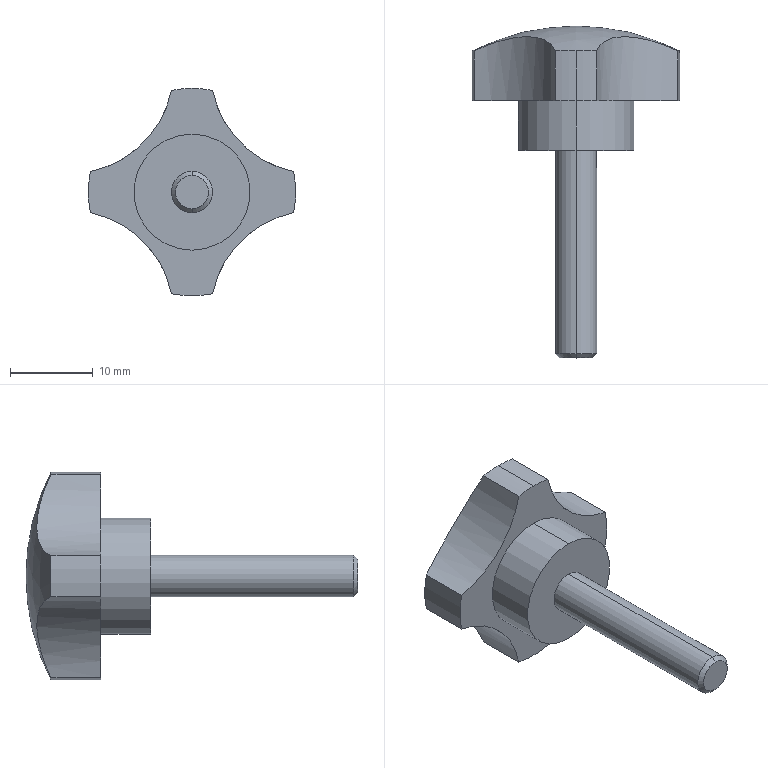Part | NX | features BREP 1 | 1 solid | 19 faces | box 25 x 40 x 25 mm | volume 4055 mm3 | cylinder 13 | plane 3 | cone 2 | sphere 1 | commonest cylinder face diameters 25 x9 5 x2 14 x2
STEP:
#1=CARTESIAN_POINT('',(12.252,12.,-2.48));
#2=VERTEX_POINT('',#1);
#3=CARTESIAN_POINT('',(12.252,12.,2.48));
#4=VERTEX_POINT('',#3);
#5=CARTESIAN_POINT('',(0.,12.,0.));
#6=DIRECTION('',(0.,-1.,0.));
#7=DIRECTION('',(0.,0.,1.));
#8=AXIS2_PLACEMENT_3D('',#5,#6,#7);
#9=CIRCLE('',#8,12.5);
#10=EDGE_CURVE('',#2,#4,#9,.T.);
#11=ORIENTED_EDGE('',*,*,#10,.F.);
#12=CARTESIAN_POINT('',(2.48,12.,-12.252));
#13=VERTEX_POINT('',#12);
#14=CARTESIAN_POINT('',(2.48,12.,-12.252));
#15=CARTESIAN_POINT('',(2.715,12.557,-11.089));
#16=CARTESIAN_POINT('',(3.495,13.393,-8.858));
#17=CARTESIAN_POINT('',(5.756,13.868,-5.744));
#18=CARTESIAN_POINT('',(8.866,13.39,-3.492));
#19=CARTESIAN_POINT('',(11.091,12.555,-2.715));
#20=CARTESIAN_POINT('',(12.252,12.,-2.48));
#21=B_SPLINE_CURVE_WITH_KNOTS('',3,(#14,#15,#16,#17,#18,#19,#20),.UNSPECIFIED.,.F.,.F.,(4,1,1,1,4),(0.,0.25,0.5,0.75,1.),.UNSPECIFIED.);
#22=EDGE_CURVE('',#2,#13,#21,.F.);
#23=ORIENTED_EDGE('',*,*,#22,.T.);
#24=CARTESIAN_POINT('',(-2.48,12.,-12.252));
#25=VERTEX_POINT('',#24);
#26=CARTESIAN_POINT('',(0.,12.,0.));
#27=DIRECTION('',(0.,-1.,0.));
#28=DIRECTION('',(0.,0.,1.));
#29=AXIS2_PLACEMENT_3D('',#26,#27,#28);
#30=CIRCLE('',#29,12.5);
#31=EDGE_CURVE('',#25,#13,#30,.T.);
#32=ORIENTED_EDGE('',*,*,#31,.F.);
#33=CARTESIAN_POINT('',(-12.252,12.,-2.48));
#34=VERTEX_POINT('',#33);
#35=CARTESIAN_POINT('',(-12.252,12.,-2.48));
#36=CARTESIAN_POINT('',(-11.089,12.557,-2.715));
#37=CARTESIAN_POINT('',(-8.858,13.393,-3.495));
#38=CARTESIAN_POINT('',(-5.744,13.868,-5.756));
#39=CARTESIAN_POINT('',(-3.492,13.39,-8.866));
#40=CARTESIAN_POINT('',(-2.715,12.555,-11.091));
#41=CARTESIAN_POINT('',(-2.48,12.,-12.252));
#42=B_SPLINE_CURVE_WITH_KNOTS('',3,(#35,#36,#37,#38,#39,#40,#41),.UNSPECIFIED.,.F.,.F.,(4,1,1,1,4),(0.,0.25,0.5,0.75,1.),.UNSPECIFIED.);
#43=EDGE_CURVE('',#25,#34,#42,.F.);
#44=ORIENTED_EDGE('',*,*,#43,.T.);
#45=CARTESIAN_POINT('',(-12.252,12.,2.48));
#46=VERTEX_POINT('',#45);
#47=CARTESIAN_POINT('',(0.,12.,0.));
#48=DIRECTION('',(0.,-1.,0.));
#49=DIRECTION('',(0.,0.,1.));
#50=AXIS2_PLACEMENT_3D('',#47,#48,#49);
#51=CIRCLE('',#50,12.5);
#52=EDGE_CURVE('',#46,#34,#51,.T.);
#53=ORIENTED_EDGE('',*,*,#52,.F.);
#54=CARTESIAN_POINT('',(-2.48,12.,12.252));
#55=VERTEX_POINT('',#54);
#56=CARTESIAN_POINT('',(-2.48,12.,12.252));
#57=CARTESIAN_POINT('',(-2.715,12.557,11.089));
#58=CARTESIAN_POINT('',(-3.495,13.393,8.858));
#59=CARTESIAN_POINT('',(-5.756,13.868,5.744));
#60=CARTESIAN_POINT('',(-8.866,13.39,3.492));
#61=CARTESIAN_POINT('',(-11.091,12.555,2.715));
#62=CARTESIAN_POINT('',(-12.252,12.,2.48));
#63=B_SPLINE_CURVE_WITH_KNOTS('',3,(#56,#57,#58,#59,#60,#61,#62),.UNSPECIFIED.,.F.,.F.,(4,1,1,1,4),(0.,0.25,0.5,0.75,1.),.UNSPECIFIED.);
#64=EDGE_CURVE('',#46,#55,#63,.F.);
#65=ORIENTED_EDGE('',*,*,#64,.T.);
#66=CARTESIAN_POINT('',(0.,12.,12.5));
#67=VERTEX_POINT('',#66);
#68=CARTESIAN_POINT('',(0.,12.,0.));
#69=DIRECTION('',(0.,-1.,0.));
#70=DIRECTION('',(0.,0.,1.));
#71=AXIS2_PLACEMENT_3D('',#68,#69,#70);
#72=CIRCLE('',#71,12.5);
#73=EDGE_CURVE('',#67,#55,#72,.T.);
#74=ORIENTED_EDGE('',*,*,#73,.F.);
#75=CARTESIAN_POINT('',(2.48,12.,12.252));
#76=VERTEX_POINT('',#75);
#77=CARTESIAN_POINT('',(0.,12.,0.));
#78=DIRECTION('',(0.,-1.,0.));
#79=DIRECTION('',(0.,0.,1.));
#80=AXIS2_PLACEMENT_3D('',#77,#78,#79);
#81=CIRCLE('',#80,12.5);
#82=EDGE_CURVE('',#76,#67,#81,.T.);
#83=ORIENTED_EDGE('',*,*,#82,.F.);
#84=CARTESIAN_POINT('',(12.252,12.,2.48));
#85=CARTESIAN_POINT('',(11.089,12.557,2.715));
#86=CARTESIAN_POINT('',(8.858,13.393,3.495));
#87=CARTESIAN_POINT('',(5.744,13.868,5.756));
#88=CARTESIAN_POINT('',(3.492,13.39,8.866));
#89=CARTESIAN_POINT('',(2.715,12.555,11.091));
#90=CARTESIAN_POINT('',(2.48,12.,12.252));
#91=B_SPLINE_CURVE_WITH_KNOTS('',3,(#84,#85,#86,#87,#88,#89,#90),.UNSPECIFIED.,.F.,.F.,(4,1,1,1,4),(0.,0.25,0.5,0.75,1.),.UNSPECIFIED.);
#92=EDGE_CURVE('',#76,#4,#91,.F.);
#93=ORIENTED_EDGE('',*,*,#92,.T.);
#94=EDGE_LOOP('',(#11,#23,#32,#44,#53,#65,#74,#83,#93));
#95=FACE_BOUND('',#94,.T.);
#96=CARTESIAN_POINT('',(0.,-12.542,0.));
#97=DIRECTION('',(1.,0.,0.));
#98=DIRECTION('',(0.,0.,-1.));
#99=AXIS2_PLACEMENT_3D('',#96,#97,#98);
#100=SPHERICAL_SURFACE('',#99,27.542);
#101=ADVANCED_FACE('',(#95),#100,.T.);
#102=CARTESIAN_POINT('',(-12.252,6.,2.48));
#103=VERTEX_POINT('',#102);
#104=CARTESIAN_POINT('',(-12.252,25.,2.48));
#105=DIRECTION('',(0.,1.,0.));
#106=VECTOR('',#105,1000.);
#107=LINE('',#104,#106);
#108=EDGE_CURVE('',#103,#46,#107,.T.);
#109=ORIENTED_EDGE('',*,*,#108,.T.);
#110=ORIENTED_EDGE('',*,*,#52,.T.);
#111=CARTESIAN_POINT('',(-12.252,6.,-2.48));
#112=VERTEX_POINT('',#111);
#113=CARTESIAN_POINT('',(-12.252,25.,-2.48));
#114=DIRECTION('',(0.,-1.,0.));
#115=VECTOR('',#114,1000.);
#116=LINE('',#113,#115);
#117=EDGE_CURVE('',#34,#112,#116,.T.);
#118=ORIENTED_EDGE('',*,*,#117,.T.);
#119=CARTESIAN_POINT('',(0.,6.,0.));
#120=DIRECTION('',(0.,1.,0.));
#121=DIRECTION('',(0.,0.,1.));
#122=AXIS2_PLACEMENT_3D('',#119,#120,#121);
#123=CIRCLE('',#122,12.5);
#124=EDGE_CURVE('',#112,#103,#123,.T.);
#125=ORIENTED_EDGE('',*,*,#124,.T.);
#126=EDGE_LOOP('',(#109,#110,#118,#125));
#127=FACE_BOUND('',#126,.T.);
#128=CARTESIAN_POINT('',(0.,0.,0.));
#129=DIRECTION('',(0.,1.,0.));
#130=DIRECTION('',(0.,0.,1.));
#131=AXIS2_PLACEMENT_3D('',#128,#129,#130);
#132=CYLINDRICAL_SURFACE('',#131,12.5);
#133=ADVANCED_FACE('',(#127),#132,.T.);
#134=CARTESIAN_POINT('',(-2.48,6.,12.252));
#135=VERTEX_POINT('',#134);
#136=CARTESIAN_POINT('',(-14.731,6.,14.731));
#137=DIRECTION('',(0.,-1.,0.));
#138=DIRECTION('',(0.,0.,1.));
#139=AXIS2_PLACEMENT_3D('',#136,#137,#138);
#140=CIRCLE('',#139,12.5);
#141=EDGE_CURVE('',#103,#135,#140,.T.);
#142=ORIENTED_EDGE('',*,*,#141,.T.);
#143=CARTESIAN_POINT('',(-2.48,0.,12.252));
#144=DIRECTION('',(0.,-1.,0.));
#145=VECTOR('',#144,1000.);
#146=LINE('',#143,#145);
#147=EDGE_CURVE('',#55,#135,#146,.T.);
#148=ORIENTED_EDGE('',*,*,#147,.F.);
#149=ORIENTED_EDGE('',*,*,#64,.F.);
#150=ORIENTED_EDGE('',*,*,#108,.F.);
#151=EDGE_LOOP('',(#142,#148,#149,#150));
#152=FACE_BOUND('',#151,.T.);
#153=CARTESIAN_POINT('',(-14.731,25.,14.731));
#154=DIRECTION('',(0.,1.,0.));
#155=DIRECTION('',(0.,0.,1.));
#156=AXIS2_PLACEMENT_3D('',#153,#154,#155);
#157=CYLINDRICAL_SURFACE('',#156,12.5);
#158=ADVANCED_FACE('',(#152),#157,.F.);
#159=CARTESIAN_POINT('',(0.,6.,12.5));
#160=VERTEX_POINT('',#159);
#161=CARTESIAN_POINT('',(0.,0.,12.5));
#162=DIRECTION('',(0.,1.,0.));
#163=VECTOR('',#162,1000.);
#164=LINE('',#161,#163);
#165=EDGE_CURVE('',#160,#67,#164,.T.);
#166=ORIENTED_EDGE('',*,*,#165,.F.);
#167=CARTESIAN_POINT('',(2.48,6.,12.252));
#168=VERTEX_POINT('',#167);
#169=CARTESIAN_POINT('',(0.,6.,0.));
#170=DIRECTION('',(0.,1.,0.));
#171=DIRECTION('',(0.,0.,1.));
#172=AXIS2_PLACEMENT_3D('',#169,#170,#171);
#173=CIRCLE('',#172,12.5);
#174=EDGE_CURVE('',#160,#168,#173,.T.);
#175=ORIENTED_EDGE('',*,*,#174,.T.);
#176=CARTESIAN_POINT('',(2.48,25.,12.252));
#177=DIRECTION('',(0.,1.,0.));
#178=VECTOR('',#177,1000.);
#179=LINE('',#176,#178);
#180=EDGE_CURVE('',#168,#76,#179,.T.);
#181=ORIENTED_EDGE('',*,*,#180,.T.);
#182=ORIENTED_EDGE('',*,*,#82,.T.);
#183=EDGE_LOOP('',(#166,#175,#181,#182));
#184=FACE_BOUND('',#183,.T.);
#185=CARTESIAN_POINT('',(0.,0.,0.));
#186=DIRECTION('',(0.,1.,0.));
#187=DIRECTION('',(0.,0.,1.));
#188=AXIS2_PLACEMENT_3D('',#185,#186,#187);
#189=CYLINDRICAL_SURFACE('',#188,12.5);
#190=ADVANCED_FACE('',(#184),#189,.T.);
#191=CARTESIAN_POINT('',(12.252,6.,2.48));
#192=VERTEX_POINT('',#191);
#193=CARTESIAN_POINT('',(14.731,6.,14.731));
#194=DIRECTION('',(0.,-1.,0.));
#195=DIRECTION('',(0.,0.,1.));
#196=AXIS2_PLACEMENT_3D('',#193,#194,#195);
#197=CIRCLE('',#196,12.5);
#198=EDGE_CURVE('',#168,#192,#197,.T.);
#199=ORIENTED_EDGE('',*,*,#198,.T.);
#200=CARTESIAN_POINT('',(12.252,0.,2.48));
#201=DIRECTION('',(0.,-1.,0.));
#202=VECTOR('',#201,1000.);
#203=LINE('',#200,#202);
#204=EDGE_CURVE('',#4,#192,#203,.T.);
#205=ORIENTED_EDGE('',*,*,#204,.F.);
#206=ORIENTED_EDGE('',*,*,#92,.F.);
#207=ORIENTED_EDGE('',*,*,#180,.F.);
#208=EDGE_LOOP('',(#199,#205,#206,#207));
#209=FACE_BOUND('',#208,.T.);
#210=CARTESIAN_POINT('',(14.731,25.,14.731));
#211=DIRECTION('',(0.,1.,0.));
#212=DIRECTION('',(0.,0.,1.));
#213=AXIS2_PLACEMENT_3D('',#210,#211,#212);
#214=CYLINDRICAL_SURFACE('',#213,12.5);
#215=ADVANCED_FACE('',(#209),#214,.F.);
#216=CARTESIAN_POINT('',(12.252,6.,-2.48));
#217=VERTEX_POINT('',#216);
#218=CARTESIAN_POINT('',(12.252,25.,-2.48));
#219=DIRECTION('',(0.,1.,0.));
#220=VECTOR('',#219,1000.);
#221=LINE('',#218,#220);
#222=EDGE_CURVE('',#217,#2,#221,.T.);
#223=ORIENTED_EDGE('',*,*,#222,.T.);
#224=ORIENTED_EDGE('',*,*,#10,.T.);
#225=ORIENTED_EDGE('',*,*,#204,.T.);
#226=CARTESIAN_POINT('',(0.,6.,0.));
#227=DIRECTION('',(0.,1.,0.));
#228=DIRECTION('',(0.,0.,1.));
#229=AXIS2_PLACEMENT_3D('',#226,#227,#228);
#230=CIRCLE('',#229,12.5);
#231=EDGE_CURVE('',#192,#217,#230,.T.);
#232=ORIENTED_EDGE('',*,*,#231,.T.);
#233=EDGE_LOOP('',(#223,#224,#225,#232));
#234=FACE_BOUND('',#233,.T.);
#235=CARTESIAN_POINT('',(0.,0.,0.));
#236=DIRECTION('',(0.,1.,0.));
#237=DIRECTION('',(0.,0.,1.));
#238=AXIS2_PLACEMENT_3D('',#235,#236,#237);
#239=CYLINDRICAL_SURFACE('',#238,12.5);
#240=ADVANCED_FACE('',(#234),#239,.T.);
#241=CARTESIAN_POINT('',(2.48,6.,-12.252));
#242=VERTEX_POINT('',#241);
#243=CARTESIAN_POINT('',(14.731,6.,-14.731));
#244=DIRECTION('',(0.,-1.,0.));
#245=DIRECTION('',(0.,0.,1.));
#246=AXIS2_PLACEMENT_3D('',#243,#244,#245);
#247=CIRCLE('',#246,12.5);
#248=EDGE_CURVE('',#217,#242,#247,.T.);
#249=ORIENTED_EDGE('',*,*,#248,.T.);
#250=CARTESIAN_POINT('',(2.48,0.,-12.252));
#251=DIRECTION('',(0.,-1.,0.));
#252=VECTOR('',#251,1000.);
#253=LINE('',#250,#252);
#254=EDGE_CURVE('',#13,#242,#253,.T.);
#255=ORIENTED_EDGE('',*,*,#254,.F.);
#256=ORIENTED_EDGE('',*,*,#22,.F.);
#257=ORIENTED_EDGE('',*,*,#222,.F.);
#258=EDGE_LOOP('',(#249,#255,#256,#257));
#259=FACE_BOUND('',#258,.T.);
#260=CARTESIAN_POINT('',(14.731,25.,-14.731));
#261=DIRECTION('',(0.,1.,0.));
#262=DIRECTION('',(0.,0.,1.));
#263=AXIS2_PLACEMENT_3D('',#260,#261,#262);
#264=CYLINDRICAL_SURFACE('',#263,12.5);
#265=ADVANCED_FACE('',(#259),#264,.F.);
#266=ORIENTED_EDGE('',*,*,#254,.T.);
#267=CARTESIAN_POINT('',(-2.48,6.,-12.252));
#268=VERTEX_POINT('',#267);
#269=CARTESIAN_POINT('',(0.,6.,0.));
#270=DIRECTION('',(0.,1.,0.));
#271=DIRECTION('',(0.,0.,1.));
#272=AXIS2_PLACEMENT_3D('',#269,#270,#271);
#273=CIRCLE('',#272,12.5);
#274=EDGE_CURVE('',#242,#268,#273,.T.);
#275=ORIENTED_EDGE('',*,*,#274,.T.);
#276=CARTESIAN_POINT('',(-2.48,25.,-12.252));
#277=DIRECTION('',(0.,1.,0.));
#278=VECTOR('',#277,1000.);
#279=LINE('',#276,#278);
#280=EDGE_CURVE('',#268,#25,#279,.T.);
#281=ORIENTED_EDGE('',*,*,#280,.T.);
#282=ORIENTED_EDGE('',*,*,#31,.T.);
#283=EDGE_LOOP('',(#266,#275,#281,#282));
#284=FACE_BOUND('',#283,.T.);
#285=CARTESIAN_POINT('',(0.,0.,0.));
#286=DIRECTION('',(0.,1.,0.));
#287=DIRECTION('',(0.,0.,1.));
#288=AXIS2_PLACEMENT_3D('',#285,#286,#287);
#289=CYLINDRICAL_SURFACE('',#288,12.5);
#290=ADVANCED_FACE('',(#284),#289,.T.);
#291=CARTESIAN_POINT('',(-14.731,6.,-14.731));
#292=DIRECTION('',(0.,-1.,0.));
#293=DIRECTION('',(0.,0.,1.));
#294=AXIS2_PLACEMENT_3D('',#291,#292,#293);
#295=CIRCLE('',#294,12.5);
#296=EDGE_CURVE('',#268,#112,#295,.T.);
#297=ORIENTED_EDGE('',*,*,#296,.T.);
#298=ORIENTED_EDGE('',*,*,#117,.F.);
#299=ORIENTED_EDGE('',*,*,#43,.F.);
#300=ORIENTED_EDGE('',*,*,#280,.F.);
#301=EDGE_LOOP('',(#297,#298,#299,#300));
#302=FACE_BOUND('',#301,.T.);
#303=CARTESIAN_POINT('',(-14.731,25.,-14.731));
#304=DIRECTION('',(0.,1.,0.));
#305=DIRECTION('',(0.,0.,1.));
#306=AXIS2_PLACEMENT_3D('',#303,#304,#305);
#307=CYLINDRICAL_SURFACE('',#306,12.5);
#308=ADVANCED_FACE('',(#302),#307,.F.);
#309=CARTESIAN_POINT('',(0.,6.,7.));
#310=VERTEX_POINT('',#309);
#311=CARTESIAN_POINT('',(0.,6.,-7.));
#312=VERTEX_POINT('',#311);
#313=CARTESIAN_POINT('',(0.,6.,0.));
#314=DIRECTION('',(0.,-1.,0.));
#315=DIRECTION('',(0.,0.,1.));
#316=AXIS2_PLACEMENT_3D('',#313,#314,#315);
#317=CIRCLE('',#316,7.);
#318=EDGE_CURVE('',#310,#312,#317,.T.);
#319=ORIENTED_EDGE('',*,*,#318,.F.);
#320=CARTESIAN_POINT('',(0.,6.,0.));
#321=DIRECTION('',(0.,-1.,0.));
#322=DIRECTION('',(0.,0.,1.));
#323=AXIS2_PLACEMENT_3D('',#320,#321,#322);
#324=CIRCLE('',#323,7.);
#325=EDGE_CURVE('',#312,#310,#324,.T.);
#326=ORIENTED_EDGE('',*,*,#325,.F.);
#327=EDGE_LOOP('',(#319,#326));
#328=FACE_BOUND('',#327,.T.);
#329=ORIENTED_EDGE('',*,*,#274,.F.);
#330=ORIENTED_EDGE('',*,*,#248,.F.);
#331=ORIENTED_EDGE('',*,*,#231,.F.);
#332=ORIENTED_EDGE('',*,*,#198,.F.);
#333=ORIENTED_EDGE('',*,*,#174,.F.);
#334=CARTESIAN_POINT('',(0.,6.,0.));
#335=DIRECTION('',(0.,1.,0.));
#336=DIRECTION('',(0.,0.,1.));
#337=AXIS2_PLACEMENT_3D('',#334,#335,#336);
#338=CIRCLE('',#337,12.5);
#339=EDGE_CURVE('',#135,#160,#338,.T.);
#340=ORIENTED_EDGE('',*,*,#339,.F.);
#341=ORIENTED_EDGE('',*,*,#141,.F.);
#342=ORIENTED_EDGE('',*,*,#124,.F.);
#343=ORIENTED_EDGE('',*,*,#296,.F.);
#344=EDGE_LOOP('',(#329,#330,#331,#332,#333,#340,#341,#342,#343));
#345=FACE_BOUND('',#344,.T.);
#346=CARTESIAN_POINT('',(12.5,6.,0.));
#347=DIRECTION('',(0.,1.,0.));
#348=DIRECTION('',(0.,0.,1.));
#349=AXIS2_PLACEMENT_3D('',#346,#347,#348);
#350=PLANE('',#349);
#351=ADVANCED_FACE('',(#328,#345),#350,.F.);
#352=CARTESIAN_POINT('',(0.,-25.,2.009));
#353=VERTEX_POINT('',#352);
#354=CARTESIAN_POINT('',(0.,-25.,-2.009));
#355=VERTEX_POINT('',#354);
#356=CARTESIAN_POINT('',(0.,-25.,0.));
#357=DIRECTION('',(0.,1.,0.));
#358=DIRECTION('',(0.,0.,1.));
#359=AXIS2_PLACEMENT_3D('',#356,#357,#358);
#360=CIRCLE('',#359,2.009);
#361=EDGE_CURVE('',#353,#355,#360,.T.);
#362=ORIENTED_EDGE('',*,*,#361,.F.);
#363=CARTESIAN_POINT('',(0.,-25.,0.));
#364=DIRECTION('',(0.,1.,0.));
#365=DIRECTION('',(0.,0.,1.));
#366=AXIS2_PLACEMENT_3D('',#363,#364,#365);
#367=CIRCLE('',#366,2.009);
#368=EDGE_CURVE('',#355,#353,#367,.T.);
#369=ORIENTED_EDGE('',*,*,#368,.F.);
#370=EDGE_LOOP('',(#362,#369));
#371=FACE_BOUND('',#370,.T.);
#372=CARTESIAN_POINT('',(2.01,-25.,0.));
#373=DIRECTION('',(0.,1.,0.));
#374=DIRECTION('',(0.,0.,1.));
#375=AXIS2_PLACEMENT_3D('',#372,#373,#374);
#376=PLANE('',#375);
#377=ADVANCED_FACE('',(#371),#376,.F.);
#378=CARTESIAN_POINT('',(0.,0.,-7.));
#379=VERTEX_POINT('',#378);
#380=CARTESIAN_POINT('',(0.,0.,-7.));
#381=DIRECTION('',(0.,1.,0.));
#382=VECTOR('',#381,1000.);
#383=LINE('',#380,#382);
#384=EDGE_CURVE('',#312,#379,#383,.F.);
#385=ORIENTED_EDGE('',*,*,#384,.T.);
#386=CARTESIAN_POINT('',(0.,0.,7.));
#387=VERTEX_POINT('',#386);
#388=CARTESIAN_POINT('',(0.,0.,0.));
#389=DIRECTION('',(0.,1.,0.));
#390=DIRECTION('',(0.,0.,1.));
#391=AXIS2_PLACEMENT_3D('',#388,#389,#390);
#392=CIRCLE('',#391,7.);
#393=EDGE_CURVE('',#379,#387,#392,.T.);
#394=ORIENTED_EDGE('',*,*,#393,.T.);
#395=CARTESIAN_POINT('',(0.,0.,7.));
#396=DIRECTION('',(0.,1.,0.));
#397=VECTOR('',#396,1000.);
#398=LINE('',#395,#397);
#399=EDGE_CURVE('',#310,#387,#398,.F.);
#400=ORIENTED_EDGE('',*,*,#399,.F.);
#401=ORIENTED_EDGE('',*,*,#318,.T.);
#402=EDGE_LOOP('',(#385,#394,#400,#401));
#403=FACE_BOUND('',#402,.T.);
#404=CARTESIAN_POINT('',(0.,0.,0.));
#405=DIRECTION('',(0.,1.,0.));
#406=DIRECTION('',(0.,0.,1.));
#407=AXIS2_PLACEMENT_3D('',#404,#405,#406);
#408=CYLINDRICAL_SURFACE('',#407,7.);
#409=ADVANCED_FACE('',(#403),#408,.T.);
#410=CARTESIAN_POINT('',(0.,-24.509,-2.5));
#411=VERTEX_POINT('',#410);
#412=CARTESIAN_POINT('',(0.,-24.509,-2.5));
#413=DIRECTION('',(0.,0.7071,-0.7071));
#414=VECTOR('',#413,1000.);
#415=LINE('',#412,#414);
#416=EDGE_CURVE('',#411,#355,#415,.F.);
#417=ORIENTED_EDGE('',*,*,#416,.T.);
#418=ORIENTED_EDGE('',*,*,#368,.T.);
#419=CARTESIAN_POINT('',(0.,-24.509,2.5));
#420=VERTEX_POINT('',#419);
#421=CARTESIAN_POINT('',(0.,-24.509,2.5));
#422=DIRECTION('',(0.,0.7071,0.7071));
#423=VECTOR('',#422,1000.);
#424=LINE('',#421,#423);
#425=EDGE_CURVE('',#420,#353,#424,.F.);
#426=ORIENTED_EDGE('',*,*,#425,.F.);
#427=CARTESIAN_POINT('',(0.,-24.509,0.));
#428=DIRECTION('',(0.,1.,0.));
#429=DIRECTION('',(0.,0.,1.));
#430=AXIS2_PLACEMENT_3D('',#427,#428,#429);
#431=CIRCLE('',#430,2.5);
#432=EDGE_CURVE('',#411,#420,#431,.T.);
#433=ORIENTED_EDGE('',*,*,#432,.F.);
#434=EDGE_LOOP('',(#417,#418,#426,#433));
#435=FACE_BOUND('',#434,.T.);
#436=CARTESIAN_POINT('',(0.,-24.509,0.));
#437=DIRECTION('',(0.,1.,0.));
#438=DIRECTION('',(0.,0.,1.));
#439=AXIS2_PLACEMENT_3D('',#436,#437,#438);
#440=CONICAL_SURFACE('',#439,2.5,0.7854);
#441=ADVANCED_FACE('',(#435),#440,.T.);
#442=CARTESIAN_POINT('',(0.,0.,2.5));
#443=VERTEX_POINT('',#442);
#444=CARTESIAN_POINT('',(0.,0.,-2.5));
#445=VERTEX_POINT('',#444);
#446=CARTESIAN_POINT('',(0.,0.,0.));
#447=DIRECTION('',(0.,-1.,0.));
#448=DIRECTION('',(0.,0.,1.));
#449=AXIS2_PLACEMENT_3D('',#446,#447,#448);
#450=CIRCLE('',#449,2.5);
#451=EDGE_CURVE('',#443,#445,#450,.T.);
#452=ORIENTED_EDGE('',*,*,#451,.F.);
#453=CARTESIAN_POINT('',(0.,0.,0.));
#454=DIRECTION('',(0.,-1.,0.));
#455=DIRECTION('',(0.,0.,1.));
#456=AXIS2_PLACEMENT_3D('',#453,#454,#455);
#457=CIRCLE('',#456,2.5);
#458=EDGE_CURVE('',#445,#443,#457,.T.);
#459=ORIENTED_EDGE('',*,*,#458,.F.);
#460=EDGE_LOOP('',(#452,#459));
#461=FACE_BOUND('',#460,.T.);
#462=CARTESIAN_POINT('',(0.,0.,0.));
#463=DIRECTION('',(0.,1.,0.));
#464=DIRECTION('',(0.,0.,1.));
#465=AXIS2_PLACEMENT_3D('',#462,#463,#464);
#466=CIRCLE('',#465,7.);
#467=EDGE_CURVE('',#387,#379,#466,.T.);
#468=ORIENTED_EDGE('',*,*,#467,.F.);
#469=ORIENTED_EDGE('',*,*,#393,.F.);
#470=EDGE_LOOP('',(#468,#469));
#471=FACE_BOUND('',#470,.T.);
#472=CARTESIAN_POINT('',(7.,0.,0.));
#473=DIRECTION('',(0.,1.,0.));
#474=DIRECTION('',(0.,0.,1.));
#475=AXIS2_PLACEMENT_3D('',#472,#473,#474);
#476=PLANE('',#475);
#477=ADVANCED_FACE('',(#461,#471),#476,.F.);
#478=CARTESIAN_POINT('',(0.,-25.,-2.5));
#479=DIRECTION('',(0.,1.,0.));
#480=VECTOR('',#479,1000.);
#481=LINE('',#478,#480);
#482=EDGE_CURVE('',#445,#411,#481,.F.);
#483=ORIENTED_EDGE('',*,*,#482,.T.);
#484=ORIENTED_EDGE('',*,*,#432,.T.);
#485=CARTESIAN_POINT('',(0.,-25.,2.5));
#486=DIRECTION('',(0.,1.,0.));
#487=VECTOR('',#486,1000.);
#488=LINE('',#485,#487);
#489=EDGE_CURVE('',#443,#420,#488,.F.);
#490=ORIENTED_EDGE('',*,*,#489,.F.);
#491=ORIENTED_EDGE('',*,*,#451,.T.);
#492=EDGE_LOOP('',(#483,#484,#490,#491));
#493=FACE_BOUND('',#492,.T.);
#494=CARTESIAN_POINT('',(0.,-25.,0.));
#495=DIRECTION('',(0.,1.,0.));
#496=DIRECTION('',(0.,0.,1.));
#497=AXIS2_PLACEMENT_3D('',#494,#495,#496);
#498=CYLINDRICAL_SURFACE('',#497,2.5);
#499=ADVANCED_FACE('',(#493),#498,.T.);
#500=ORIENTED_EDGE('',*,*,#339,.T.);
#501=ORIENTED_EDGE('',*,*,#165,.T.);
#502=ORIENTED_EDGE('',*,*,#73,.T.);
#503=ORIENTED_EDGE('',*,*,#147,.T.);
#504=EDGE_LOOP('',(#500,#501,#502,#503));
#505=FACE_BOUND('',#504,.T.);
#506=CARTESIAN_POINT('',(0.,0.,0.));
#507=DIRECTION('',(0.,1.,0.));
#508=DIRECTION('',(0.,0.,1.));
#509=AXIS2_PLACEMENT_3D('',#506,#507,#508);
#510=CYLINDRICAL_SURFACE('',#509,12.5);
#511=ADVANCED_FACE('',(#505),#510,.T.);
#512=ORIENTED_EDGE('',*,*,#467,.T.);
#513=ORIENTED_EDGE('',*,*,#384,.F.);
#514=ORIENTED_EDGE('',*,*,#325,.T.);
#515=ORIENTED_EDGE('',*,*,#399,.T.);
#516=EDGE_LOOP('',(#512,#513,#514,#515));
#517=FACE_BOUND('',#516,.T.);
#518=CARTESIAN_POINT('',(0.,0.,0.));
#519=DIRECTION('',(0.,1.,0.));
#520=DIRECTION('',(0.,0.,1.));
#521=AXIS2_PLACEMENT_3D('',#518,#519,#520);
#522=CYLINDRICAL_SURFACE('',#521,7.);
#523=ADVANCED_FACE('',(#517),#522,.T.);
#524=ORIENTED_EDGE('',*,*,#361,.T.);
#525=ORIENTED_EDGE('',*,*,#416,.F.);
#526=CARTESIAN_POINT('',(0.,-24.509,0.));
#527=DIRECTION('',(0.,1.,0.));
#528=DIRECTION('',(0.,0.,1.));
#529=AXIS2_PLACEMENT_3D('',#526,#527,#528);
#530=CIRCLE('',#529,2.5);
#531=EDGE_CURVE('',#420,#411,#530,.T.);
#532=ORIENTED_EDGE('',*,*,#531,.F.);
#533=ORIENTED_EDGE('',*,*,#425,.T.);
#534=EDGE_LOOP('',(#524,#525,#532,#533));
#535=FACE_BOUND('',#534,.T.);
#536=CARTESIAN_POINT('',(0.,-24.509,0.));
#537=DIRECTION('',(0.,1.,0.));
#538=DIRECTION('',(0.,0.,1.));
#539=AXIS2_PLACEMENT_3D('',#536,#537,#538);
#540=CONICAL_SURFACE('',#539,2.5,0.7854);
#541=ADVANCED_FACE('',(#535),#540,.T.);
#542=ORIENTED_EDGE('',*,*,#531,.T.);
#543=ORIENTED_EDGE('',*,*,#482,.F.);
#544=ORIENTED_EDGE('',*,*,#458,.T.);
#545=ORIENTED_EDGE('',*,*,#489,.T.);
#546=EDGE_LOOP('',(#542,#543,#544,#545));
#547=FACE_BOUND('',#546,.T.);
#548=CARTESIAN_POINT('',(0.,-25.,0.));
#549=DIRECTION('',(0.,1.,0.));
#550=DIRECTION('',(0.,0.,1.));
#551=AXIS2_PLACEMENT_3D('',#548,#549,#550);
#552=CYLINDRICAL_SURFACE('',#551,2.5);
#553=ADVANCED_FACE('',(#547),#552,.T.);
#554=CLOSED_SHELL('',(#101,#133,#158,#190,#215,#240,#265,#290,#308,#351,#377,#409,#441,#477,#499,#511,#523,#541,#553));
#555=MANIFOLD_SOLID_BREP('',#554);
#556=(LENGTH_UNIT()NAMED_UNIT(*)SI_UNIT(.MILLI.,.METRE.));
#557=UNCERTAINTY_MEASURE_WITH_UNIT(LENGTH_MEASURE(0.0508),#556,'','');
#558=(NAMED_UNIT(*)PLANE_ANGLE_UNIT()SI_UNIT($,.RADIAN.));
#559=(NAMED_UNIT(*)SI_UNIT($,.STERADIAN.)SOLID_ANGLE_UNIT());
#560=(GEOMETRIC_REPRESENTATION_CONTEXT(3)GLOBAL_UNCERTAINTY_ASSIGNED_CONTEXT((#557))GLOBAL_UNIT_ASSIGNED_CONTEXT((#556,#558,#559))REPRESENTATION_CONTEXT('',''));
#561=ADVANCED_BREP_SHAPE_REPRESENTATION('',(#555),#560);